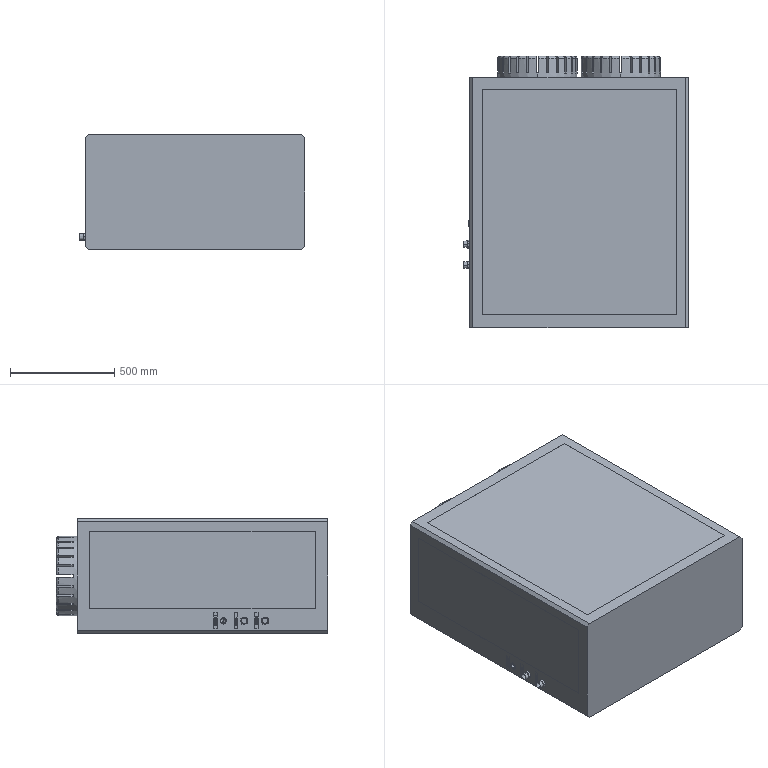Part | SolidWorks | features ICE 14, LPattern 2, Chamfer 1, CirPattern 1, Extrusion 1, Fillet 1, HoleWzd 1 | 1 solid | 1390 faces | box 1080 x 1300 x 550.2 mm | volume 708299280 mm3 | plane 1228 | spline 92 | torus 48 | cylinder 12 | cone 10 | commonest cylinder face diameters 80 x4 380 x4 24.5 x2 30.5 x2